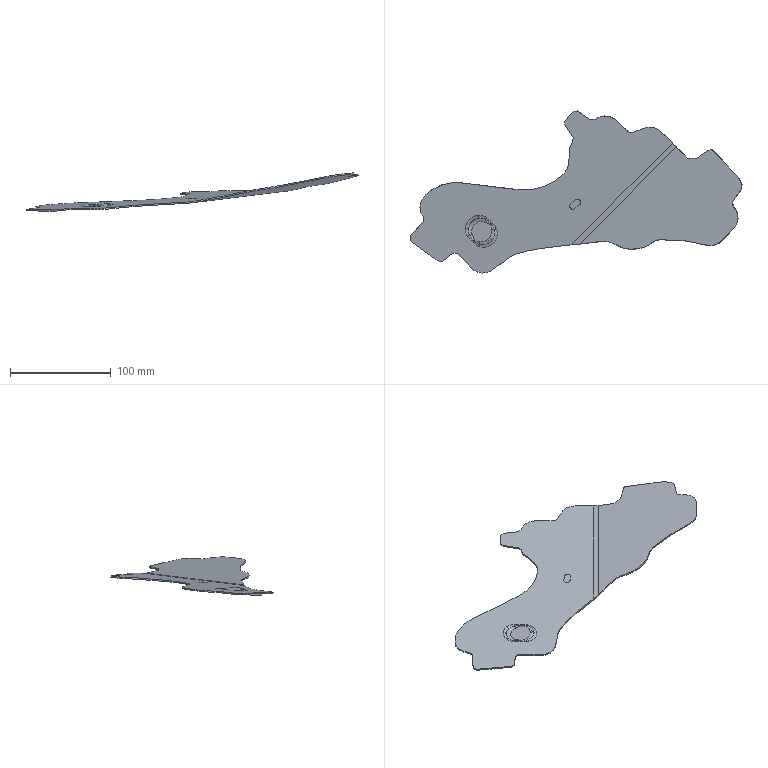Part | STEP file | 9805823380.1BPIECE_SOLIDE_FINALE_id1042_x_t | 1 solid | 118 faces | box 329.111 x 160.705 x 37.841 mm | volume 35454 mm3 | spline 100 | plane 15 | cylinder 3 | commonest cylinder face diameters 3 x1 54 x1 56.5 x1